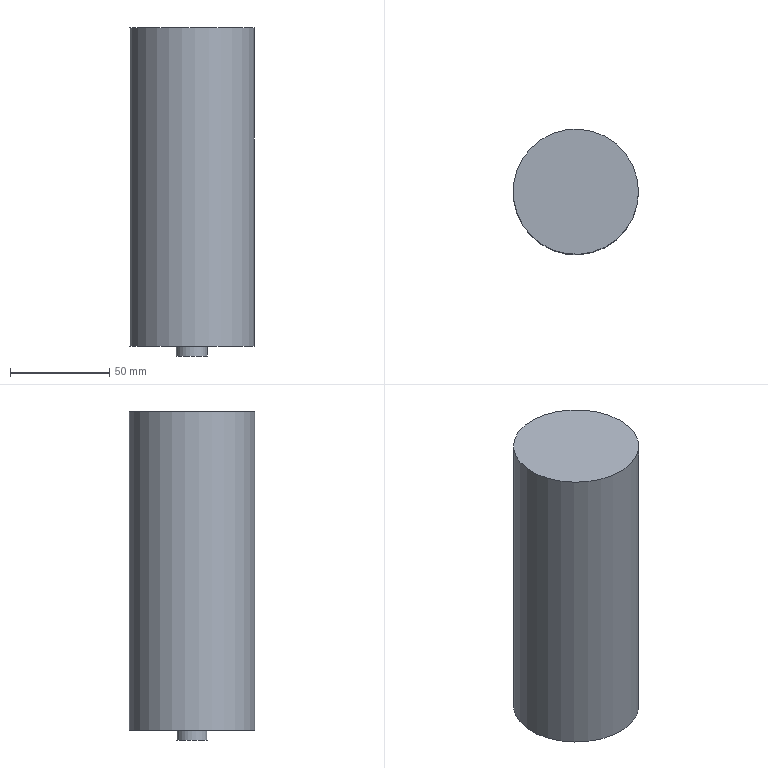Part | NX | features solid 2 | 1 solid | 5 faces | box 63 x 63 x 165 mm | volume 499703 mm3 | plane 3 | cylinder 2 | commonest cylinder face diameters 15.5 x1 63 x1
STEP:
#1=CARTESIAN_POINT('',(1923.,288.5,30.));
#2=VERTEX_POINT('',#1);
#3=CARTESIAN_POINT('',(1891.5,288.5,30.));
#4=DIRECTION('',(0.,0.,1.));
#5=DIRECTION('',(1.,0.,0.));
#6=AXIS2_PLACEMENT_3D('',#3,#4,#5);
#7=CIRCLE('',#6,31.5);
#8=EDGE_CURVE('',#2,#2,#7,.T.);
#9=ORIENTED_EDGE('',*,*,#8,.F.);
#10=EDGE_LOOP('',(#9));
#11=FACE_BOUND('',#10,.T.);
#12=CARTESIAN_POINT('',(1899.25,288.5,30.));
#13=VERTEX_POINT('',#12);
#14=CARTESIAN_POINT('',(1891.5,288.5,30.));
#15=DIRECTION('',(0.,0.,1.));
#16=DIRECTION('',(1.,0.,0.));
#17=AXIS2_PLACEMENT_3D('',#14,#15,#16);
#18=CIRCLE('',#17,7.75);
#19=EDGE_CURVE('',#13,#13,#18,.F.);
#20=ORIENTED_EDGE('',*,*,#19,.F.);
#21=EDGE_LOOP('',(#20));
#22=FACE_BOUND('',#21,.T.);
#23=CARTESIAN_POINT('',(1891.5,288.5,30.));
#24=DIRECTION('',(0.,0.,1.));
#25=DIRECTION('',(1.,0.,0.));
#26=AXIS2_PLACEMENT_3D('',#23,#24,#25);
#27=PLANE('',#26);
#28=ADVANCED_FACE('',(#11,#22),#27,.F.);
#29=CARTESIAN_POINT('',(1923.,288.5,190.));
#30=VERTEX_POINT('',#29);
#31=CARTESIAN_POINT('',(1891.5,288.5,190.));
#32=DIRECTION('',(0.,0.,1.));
#33=DIRECTION('',(1.,0.,0.));
#34=AXIS2_PLACEMENT_3D('',#31,#32,#33);
#35=CIRCLE('',#34,31.5);
#36=EDGE_CURVE('',#30,#30,#35,.T.);
#37=ORIENTED_EDGE('',*,*,#36,.F.);
#38=EDGE_LOOP('',(#37));
#39=FACE_BOUND('',#38,.T.);
#40=ORIENTED_EDGE('',*,*,#8,.T.);
#41=EDGE_LOOP('',(#40));
#42=FACE_BOUND('',#41,.T.);
#43=CARTESIAN_POINT('',(1891.5,288.5,190.));
#44=DIRECTION('',(0.,0.,-1.));
#45=DIRECTION('',(-1.,0.,0.));
#46=AXIS2_PLACEMENT_3D('',#43,#44,#45);
#47=CYLINDRICAL_SURFACE('',#46,31.5);
#48=ADVANCED_FACE('',(#39,#42),#47,.T.);
#49=ORIENTED_EDGE('',*,*,#36,.T.);
#50=EDGE_LOOP('',(#49));
#51=FACE_BOUND('',#50,.T.);
#52=CARTESIAN_POINT('',(1891.5,288.5,190.));
#53=DIRECTION('',(0.,0.,1.));
#54=DIRECTION('',(1.,0.,0.));
#55=AXIS2_PLACEMENT_3D('',#52,#53,#54);
#56=PLANE('',#55);
#57=ADVANCED_FACE('',(#51),#56,.T.);
#58=CARTESIAN_POINT('',(1883.75,288.5,25.));
#59=VERTEX_POINT('',#58);
#60=CARTESIAN_POINT('',(1891.5,288.5,25.));
#61=DIRECTION('',(0.,0.,-1.));
#62=DIRECTION('',(-1.,0.,0.));
#63=AXIS2_PLACEMENT_3D('',#60,#61,#62);
#64=CIRCLE('',#63,7.75);
#65=EDGE_CURVE('',#59,#59,#64,.T.);
#66=ORIENTED_EDGE('',*,*,#65,.F.);
#67=EDGE_LOOP('',(#66));
#68=FACE_BOUND('',#67,.T.);
#69=ORIENTED_EDGE('',*,*,#19,.T.);
#70=EDGE_LOOP('',(#69));
#71=FACE_BOUND('',#70,.T.);
#72=CARTESIAN_POINT('',(1891.5,288.5,25.));
#73=DIRECTION('',(0.,0.,1.));
#74=DIRECTION('',(1.,0.,0.));
#75=AXIS2_PLACEMENT_3D('',#72,#73,#74);
#76=CYLINDRICAL_SURFACE('',#75,7.75);
#77=ADVANCED_FACE('',(#68,#71),#76,.T.);
#78=ORIENTED_EDGE('',*,*,#65,.T.);
#79=EDGE_LOOP('',(#78));
#80=FACE_BOUND('',#79,.T.);
#81=CARTESIAN_POINT('',(1891.5,288.5,25.));
#82=DIRECTION('',(0.,0.,-1.));
#83=DIRECTION('',(-1.,0.,0.));
#84=AXIS2_PLACEMENT_3D('',#81,#82,#83);
#85=PLANE('',#84);
#86=ADVANCED_FACE('',(#80),#85,.T.);
#87=CLOSED_SHELL('',(#28,#48,#57,#77,#86));
#88=MANIFOLD_SOLID_BREP('',#87);
#89=(LENGTH_UNIT()NAMED_UNIT(*)SI_UNIT(.MILLI.,.METRE.));
#90=UNCERTAINTY_MEASURE_WITH_UNIT(LENGTH_MEASURE(0.00001),#89,'','');
#91=(NAMED_UNIT(*)PLANE_ANGLE_UNIT()SI_UNIT($,.RADIAN.));
#92=(NAMED_UNIT(*)SI_UNIT($,.STERADIAN.)SOLID_ANGLE_UNIT());
#93=(GEOMETRIC_REPRESENTATION_CONTEXT(3)GLOBAL_UNCERTAINTY_ASSIGNED_CONTEXT((#90))GLOBAL_UNIT_ASSIGNED_CONTEXT((#89,#91,#92))REPRESENTATION_CONTEXT('',''));
#94=ADVANCED_BREP_SHAPE_REPRESENTATION('',(#88),#93);